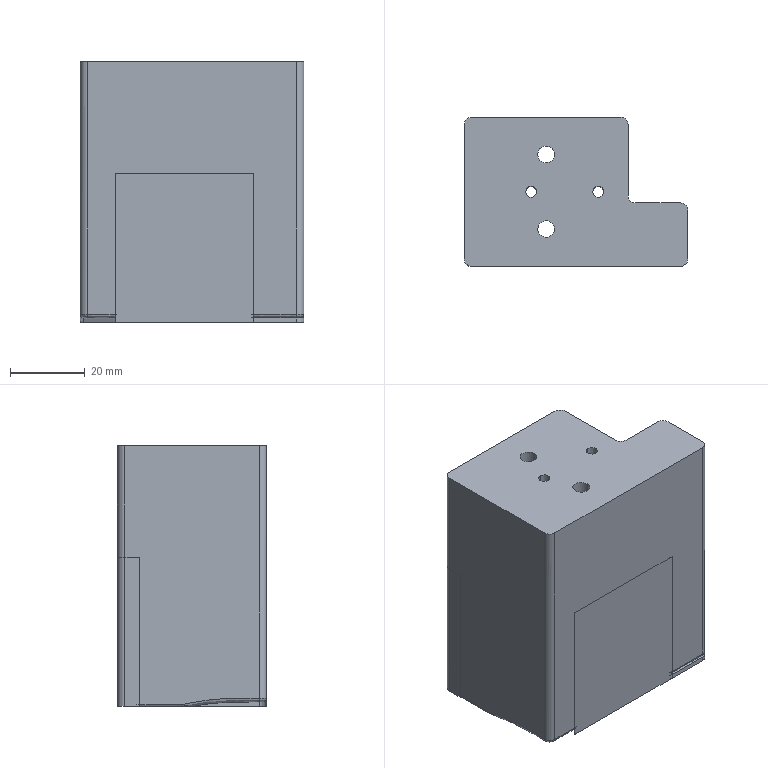Part | 3 solids | 100 faces | box 60.004 x 40.015 x 70 mm | volume 134761 mm3 | cylinder 39 | spline 35 | plane 23 | torus 3 | commonest cylinder face diameters 4 x17 3 x6 8 x6 4.5 x4 10 x4 1 x2